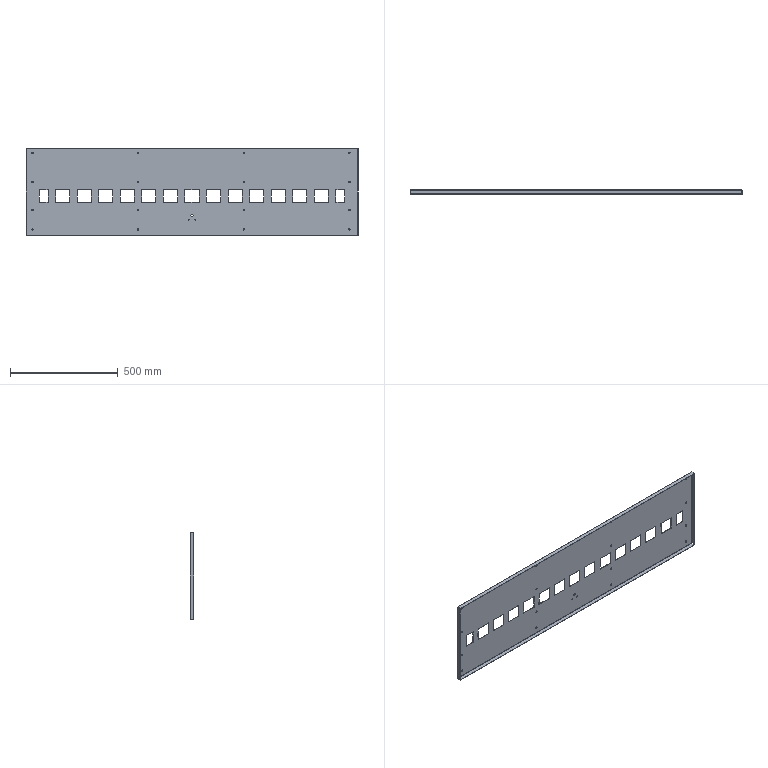Part | SolidWorks | features ICE 4, HoleWzd 2, LPattern 2, EdgeFlange 1, FlatPattern 1, SMBaseFlange 1, SheetMetal 1 | 1 solid | 136 faces | box 1540 x 18.5 x 407 mm | volume 949433 mm3 | plane 82 | cone 36 | cylinder 10 | spline 8 | commonest cylinder face diameters 1.473 x4 4.473 x4 10 x2